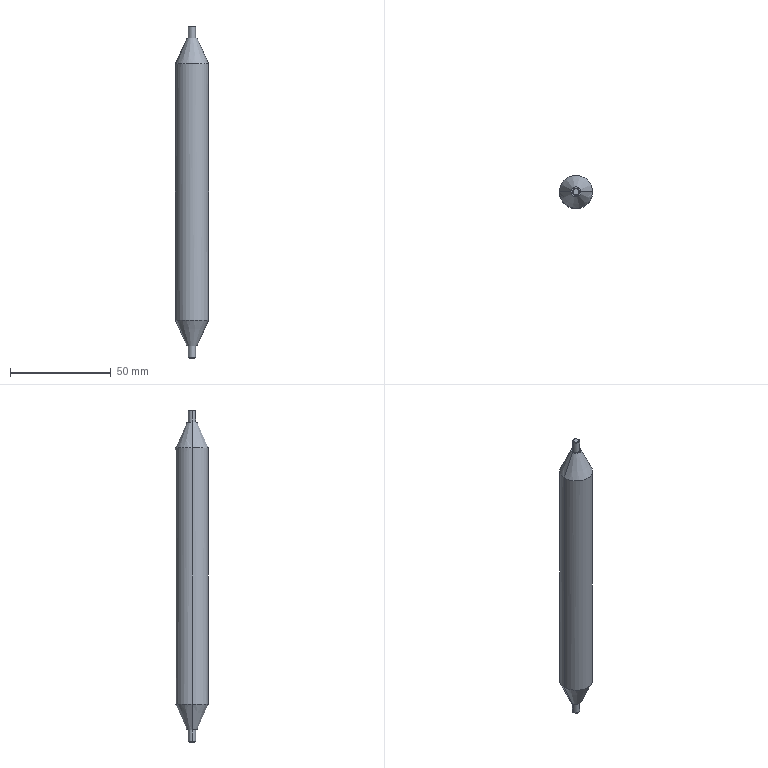Part | SolidWorks | features MirrorPattern 2, StudWizard 2, Blend 1, Extrusion 1, ICE 1 | 1 solid | 22 faces | box 16.35 x 16.35 x 164.4 mm | volume 13178 mm3 | cone 8 | cylinder 8 | plane 6 | commonest cylinder face diameters 3.5 x4 12.7 x2 16.35 x2
STEP:
#1=CARTESIAN_POINT('',(-1.414,0.,82.2));
#2=VERTEX_POINT('',#1);
#3=CARTESIAN_POINT('',(1.414,0.,82.2));
#4=VERTEX_POINT('',#3);
#5=CARTESIAN_POINT('',(0.,0.,82.2));
#6=DIRECTION('',(0.,0.,-1.));
#7=DIRECTION('',(-1.,0.,0.));
#8=AXIS2_PLACEMENT_3D('',#5,#6,#7);
#9=CIRCLE('',#8,1.414);
#10=EDGE_CURVE('',#2,#4,#9,.T.);
#11=ORIENTED_EDGE('',*,*,#10,.T.);
#12=CARTESIAN_POINT('',(1.75,0.,81.865));
#13=VERTEX_POINT('',#12);
#14=CARTESIAN_POINT('',(1.414,0.,82.2));
#15=DIRECTION('',(0.7071,0.,-0.7071));
#16=VECTOR('',#15,1000.);
#17=LINE('',#14,#16);
#18=EDGE_CURVE('',#4,#13,#17,.T.);
#19=ORIENTED_EDGE('',*,*,#18,.T.);
#20=CARTESIAN_POINT('',(-1.75,0.,81.865));
#21=VERTEX_POINT('',#20);
#22=CARTESIAN_POINT('',(0.,0.,81.865));
#23=DIRECTION('',(0.,0.,-1.));
#24=DIRECTION('',(-1.,0.,0.));
#25=AXIS2_PLACEMENT_3D('',#22,#23,#24);
#26=CIRCLE('',#25,1.75);
#27=EDGE_CURVE('',#21,#13,#26,.T.);
#28=ORIENTED_EDGE('',*,*,#27,.F.);
#29=CARTESIAN_POINT('',(-1.414,0.,82.2));
#30=DIRECTION('',(-0.7071,0.,-0.7071));
#31=VECTOR('',#30,1000.);
#32=LINE('',#29,#31);
#33=EDGE_CURVE('',#2,#21,#32,.T.);
#34=ORIENTED_EDGE('',*,*,#33,.F.);
#35=EDGE_LOOP('',(#11,#19,#28,#34));
#36=FACE_OUTER_BOUND('',#35,.T.);
#37=CARTESIAN_POINT('',(0.,0.,82.2));
#38=DIRECTION('',(0.,0.,-1.));
#39=DIRECTION('',(-1.,0.,0.));
#40=AXIS2_PLACEMENT_3D('',#37,#38,#39);
#41=CONICAL_SURFACE('',#40,1.414,0.7854);
#42=ADVANCED_FACE('',(#36),#41,.T.);
#43=ORIENTED_EDGE('',*,*,#27,.T.);
#44=CARTESIAN_POINT('',(1.75,0.,76.2));
#45=VERTEX_POINT('',#44);
#46=CARTESIAN_POINT('',(1.75,0.,82.2));
#47=DIRECTION('',(0.,0.,-1.));
#48=VECTOR('',#47,1000.);
#49=LINE('',#46,#48);
#50=EDGE_CURVE('',#13,#45,#49,.T.);
#51=ORIENTED_EDGE('',*,*,#50,.T.);
#52=CARTESIAN_POINT('',(-1.75,0.,76.2));
#53=VERTEX_POINT('',#52);
#54=CARTESIAN_POINT('',(0.,0.,76.2));
#55=DIRECTION('',(0.,0.,-1.));
#56=DIRECTION('',(-1.,0.,0.));
#57=AXIS2_PLACEMENT_3D('',#54,#55,#56);
#58=CIRCLE('',#57,1.75);
#59=EDGE_CURVE('',#53,#45,#58,.T.);
#60=ORIENTED_EDGE('',*,*,#59,.F.);
#61=CARTESIAN_POINT('',(-1.75,0.,82.2));
#62=DIRECTION('',(0.,0.,-1.));
#63=VECTOR('',#62,1000.);
#64=LINE('',#61,#63);
#65=EDGE_CURVE('',#21,#53,#64,.T.);
#66=ORIENTED_EDGE('',*,*,#65,.F.);
#67=EDGE_LOOP('',(#43,#51,#60,#66));
#68=FACE_OUTER_BOUND('',#67,.T.);
#69=CARTESIAN_POINT('',(0.,0.,82.2));
#70=DIRECTION('',(0.,0.,-1.));
#71=DIRECTION('',(-1.,0.,0.));
#72=AXIS2_PLACEMENT_3D('',#69,#70,#71);
#73=CYLINDRICAL_SURFACE('',#72,1.75);
#74=ADVANCED_FACE('',(#68),#73,.T.);
#75=CARTESIAN_POINT('',(1.414,0.,-82.2));
#76=VERTEX_POINT('',#75);
#77=CARTESIAN_POINT('',(-1.414,0.,-82.2));
#78=VERTEX_POINT('',#77);
#79=CARTESIAN_POINT('',(0.,0.,-82.2));
#80=DIRECTION('',(0.,0.,1.));
#81=DIRECTION('',(1.,0.,0.));
#82=AXIS2_PLACEMENT_3D('',#79,#80,#81);
#83=CIRCLE('',#82,1.414);
#84=EDGE_CURVE('',#76,#78,#83,.T.);
#85=ORIENTED_EDGE('',*,*,#84,.T.);
#86=CARTESIAN_POINT('',(-1.75,0.,-81.865));
#87=VERTEX_POINT('',#86);
#88=CARTESIAN_POINT('',(-1.414,0.,-82.2));
#89=DIRECTION('',(-0.7071,0.,0.7071));
#90=VECTOR('',#89,1000.);
#91=LINE('',#88,#90);
#92=EDGE_CURVE('',#78,#87,#91,.T.);
#93=ORIENTED_EDGE('',*,*,#92,.T.);
#94=CARTESIAN_POINT('',(1.75,0.,-81.865));
#95=VERTEX_POINT('',#94);
#96=CARTESIAN_POINT('',(0.,0.,-81.865));
#97=DIRECTION('',(0.,0.,1.));
#98=DIRECTION('',(1.,0.,0.));
#99=AXIS2_PLACEMENT_3D('',#96,#97,#98);
#100=CIRCLE('',#99,1.75);
#101=EDGE_CURVE('',#95,#87,#100,.T.);
#102=ORIENTED_EDGE('',*,*,#101,.F.);
#103=CARTESIAN_POINT('',(1.414,0.,-82.2));
#104=DIRECTION('',(0.7071,0.,0.7071));
#105=VECTOR('',#104,1000.);
#106=LINE('',#103,#105);
#107=EDGE_CURVE('',#76,#95,#106,.T.);
#108=ORIENTED_EDGE('',*,*,#107,.F.);
#109=EDGE_LOOP('',(#85,#93,#102,#108));
#110=FACE_OUTER_BOUND('',#109,.T.);
#111=CARTESIAN_POINT('',(0.,0.,-82.2));
#112=DIRECTION('',(0.,0.,1.));
#113=DIRECTION('',(1.,0.,0.));
#114=AXIS2_PLACEMENT_3D('',#111,#112,#113);
#115=CONICAL_SURFACE('',#114,1.414,0.7854);
#116=ADVANCED_FACE('',(#110),#115,.T.);
#117=ORIENTED_EDGE('',*,*,#101,.T.);
#118=CARTESIAN_POINT('',(-1.75,0.,-76.2));
#119=VERTEX_POINT('',#118);
#120=CARTESIAN_POINT('',(-1.75,0.,-82.2));
#121=DIRECTION('',(0.,0.,1.));
#122=VECTOR('',#121,1000.);
#123=LINE('',#120,#122);
#124=EDGE_CURVE('',#87,#119,#123,.T.);
#125=ORIENTED_EDGE('',*,*,#124,.T.);
#126=CARTESIAN_POINT('',(1.75,0.,-76.2));
#127=VERTEX_POINT('',#126);
#128=CARTESIAN_POINT('',(0.,0.,-76.2));
#129=DIRECTION('',(0.,0.,1.));
#130=DIRECTION('',(1.,0.,0.));
#131=AXIS2_PLACEMENT_3D('',#128,#129,#130);
#132=CIRCLE('',#131,1.75);
#133=EDGE_CURVE('',#127,#119,#132,.T.);
#134=ORIENTED_EDGE('',*,*,#133,.F.);
#135=CARTESIAN_POINT('',(1.75,0.,-82.2));
#136=DIRECTION('',(0.,0.,1.));
#137=VECTOR('',#136,1000.);
#138=LINE('',#135,#137);
#139=EDGE_CURVE('',#95,#127,#138,.T.);
#140=ORIENTED_EDGE('',*,*,#139,.F.);
#141=EDGE_LOOP('',(#117,#125,#134,#140));
#142=FACE_OUTER_BOUND('',#141,.T.);
#143=CARTESIAN_POINT('',(0.,0.,-82.2));
#144=DIRECTION('',(0.,0.,1.));
#145=DIRECTION('',(1.,0.,0.));
#146=AXIS2_PLACEMENT_3D('',#143,#144,#145);
#147=CYLINDRICAL_SURFACE('',#146,1.75);
#148=ADVANCED_FACE('',(#142),#147,.T.);
#149=CARTESIAN_POINT('',(2.5,0.,76.2));
#150=VERTEX_POINT('',#149);
#151=CARTESIAN_POINT('',(-2.5,0.,76.2));
#152=VERTEX_POINT('',#151);
#153=CARTESIAN_POINT('',(2.5,0.,76.2));
#154=CARTESIAN_POINT('',(2.5,-0.3272,76.2));
#155=CARTESIAN_POINT('',(2.435,-0.6544,76.2));
#156=CARTESIAN_POINT('',(2.184,-1.259,76.2));
#157=CARTESIAN_POINT('',(1.999,-1.536,76.2));
#158=CARTESIAN_POINT('',(1.536,-1.999,76.2));
#159=CARTESIAN_POINT('',(1.259,-2.184,76.2));
#160=CARTESIAN_POINT('',(0.6544,-2.435,76.2));
#161=CARTESIAN_POINT('',(0.3272,-2.5,76.2));
#162=CARTESIAN_POINT('',(-0.3272,-2.5,76.2));
#163=CARTESIAN_POINT('',(-0.6544,-2.435,76.2));
#164=CARTESIAN_POINT('',(-1.259,-2.184,76.2));
#165=CARTESIAN_POINT('',(-1.536,-1.999,76.2));
#166=CARTESIAN_POINT('',(-1.999,-1.536,76.2));
#167=CARTESIAN_POINT('',(-2.184,-1.259,76.2));
#168=CARTESIAN_POINT('',(-2.435,-0.6544,76.2));
#169=CARTESIAN_POINT('',(-2.5,-0.3272,76.2));
#170=CARTESIAN_POINT('',(-2.5,0.,76.2));
#171=B_SPLINE_CURVE_WITH_KNOTS('',3,(#153,#154,#155,#156,#157,#158,#159,#160,#161,#162,#163,#164,#165,#166,#167,#168,#169,#170),.UNSPECIFIED.,.F.,.F.,(4,2,2,2,2,2,2,2,4),(0.,0.0625,0.125,0.1875,0.25,0.3125,0.375,0.4375,0.5),.UNSPECIFIED.);
#172=EDGE_CURVE('',#150,#152,#171,.T.);
#173=ORIENTED_EDGE('',*,*,#172,.T.);
#174=CARTESIAN_POINT('',(-8.175,0.,63.5));
#175=VERTEX_POINT('',#174);
#176=CARTESIAN_POINT('',(-2.5,0.,76.2));
#177=DIRECTION('',(-0.408,0.,-0.913));
#178=VECTOR('',#177,1000.);
#179=LINE('',#176,#178);
#180=EDGE_CURVE('',#152,#175,#179,.T.);
#181=ORIENTED_EDGE('',*,*,#180,.T.);
#182=CARTESIAN_POINT('',(8.175,0.,63.5));
#183=VERTEX_POINT('',#182);
#184=CARTESIAN_POINT('',(-8.175,0.,63.5));
#185=CARTESIAN_POINT('',(-8.175,-1.07,63.5));
#186=CARTESIAN_POINT('',(-7.962,-2.14,63.5));
#187=CARTESIAN_POINT('',(-7.143,-4.117,63.5));
#188=CARTESIAN_POINT('',(-6.537,-5.024,63.5));
#189=CARTESIAN_POINT('',(-5.024,-6.537,63.5));
#190=CARTESIAN_POINT('',(-4.117,-7.143,63.5));
#191=CARTESIAN_POINT('',(-2.14,-7.962,63.5));
#192=CARTESIAN_POINT('',(-1.07,-8.175,63.5));
#193=CARTESIAN_POINT('',(1.07,-8.175,63.5));
#194=CARTESIAN_POINT('',(2.14,-7.962,63.5));
#195=CARTESIAN_POINT('',(4.117,-7.143,63.5));
#196=CARTESIAN_POINT('',(5.024,-6.537,63.5));
#197=CARTESIAN_POINT('',(6.537,-5.024,63.5));
#198=CARTESIAN_POINT('',(7.143,-4.117,63.5));
#199=CARTESIAN_POINT('',(7.962,-2.14,63.5));
#200=CARTESIAN_POINT('',(8.175,-1.07,63.5));
#201=CARTESIAN_POINT('',(8.175,0.,63.5));
#202=B_SPLINE_CURVE_WITH_KNOTS('',3,(#184,#185,#186,#187,#188,#189,#190,#191,#192,#193,#194,#195,#196,#197,#198,#199,#200,#201),.UNSPECIFIED.,.F.,.F.,(4,2,2,2,2,2,2,2,4),(0.,0.0625,0.125,0.1875,0.25,0.3125,0.375,0.4375,0.5),.UNSPECIFIED.);
#203=EDGE_CURVE('',#175,#183,#202,.T.);
#204=ORIENTED_EDGE('',*,*,#203,.T.);
#205=CARTESIAN_POINT('',(2.5,0.,76.2));
#206=DIRECTION('',(0.408,0.,-0.913));
#207=VECTOR('',#206,1000.);
#208=LINE('',#205,#207);
#209=EDGE_CURVE('',#150,#183,#208,.T.);
#210=ORIENTED_EDGE('',*,*,#209,.F.);
#211=EDGE_LOOP('',(#173,#181,#204,#210));
#212=FACE_OUTER_BOUND('',#211,.T.);
#213=CARTESIAN_POINT('',(0.,0.,76.2));
#214=DIRECTION('',(0.,0.,-1.));
#215=DIRECTION('',(1.,0.,0.));
#216=AXIS2_PLACEMENT_3D('',#213,#214,#215);
#217=CONICAL_SURFACE('',#216,2.5,0.4202);
#218=ADVANCED_FACE('',(#212),#217,.T.);
#219=CARTESIAN_POINT('',(2.5,0.,-76.2));
#220=VERTEX_POINT('',#219);
#221=CARTESIAN_POINT('',(-2.5,0.,-76.2));
#222=VERTEX_POINT('',#221);
#223=CARTESIAN_POINT('',(2.5,0.,-76.2));
#224=CARTESIAN_POINT('',(2.5,0.3272,-76.2));
#225=CARTESIAN_POINT('',(2.435,0.6544,-76.2));
#226=CARTESIAN_POINT('',(2.184,1.259,-76.2));
#227=CARTESIAN_POINT('',(1.999,1.536,-76.2));
#228=CARTESIAN_POINT('',(1.536,1.999,-76.2));
#229=CARTESIAN_POINT('',(1.259,2.184,-76.2));
#230=CARTESIAN_POINT('',(0.6544,2.435,-76.2));
#231=CARTESIAN_POINT('',(0.3272,2.5,-76.2));
#232=CARTESIAN_POINT('',(-0.3272,2.5,-76.2));
#233=CARTESIAN_POINT('',(-0.6544,2.435,-76.2));
#234=CARTESIAN_POINT('',(-1.259,2.184,-76.2));
#235=CARTESIAN_POINT('',(-1.536,1.999,-76.2));
#236=CARTESIAN_POINT('',(-1.999,1.536,-76.2));
#237=CARTESIAN_POINT('',(-2.184,1.259,-76.2));
#238=CARTESIAN_POINT('',(-2.435,0.6544,-76.2));
#239=CARTESIAN_POINT('',(-2.5,0.3272,-76.2));
#240=CARTESIAN_POINT('',(-2.5,0.,-76.2));
#241=B_SPLINE_CURVE_WITH_KNOTS('',3,(#223,#224,#225,#226,#227,#228,#229,#230,#231,#232,#233,#234,#235,#236,#237,#238,#239,#240),.UNSPECIFIED.,.F.,.F.,(4,2,2,2,2,2,2,2,4),(0.,0.0625,0.125,0.1875,0.25,0.3125,0.375,0.4375,0.5),.UNSPECIFIED.);
#242=EDGE_CURVE('',#220,#222,#241,.T.);
#243=ORIENTED_EDGE('',*,*,#242,.T.);
#244=CARTESIAN_POINT('',(-8.175,0.,-63.5));
#245=VERTEX_POINT('',#244);
#246=CARTESIAN_POINT('',(-2.5,0.,-76.2));
#247=DIRECTION('',(-0.408,0.,0.913));
#248=VECTOR('',#247,1000.);
#249=LINE('',#246,#248);
#250=EDGE_CURVE('',#222,#245,#249,.T.);
#251=ORIENTED_EDGE('',*,*,#250,.T.);
#252=CARTESIAN_POINT('',(8.175,0.,-63.5));
#253=VERTEX_POINT('',#252);
#254=CARTESIAN_POINT('',(0.,0.,-63.5));
#255=DIRECTION('',(0.,0.,-1.));
#256=DIRECTION('',(-1.,0.,0.));
#257=AXIS2_PLACEMENT_3D('',#254,#255,#256);
#258=CIRCLE('',#257,8.175);
#259=EDGE_CURVE('',#245,#253,#258,.T.);
#260=ORIENTED_EDGE('',*,*,#259,.T.);
#261=CARTESIAN_POINT('',(2.5,0.,-76.2));
#262=DIRECTION('',(0.408,0.,0.913));
#263=VECTOR('',#262,1000.);
#264=LINE('',#261,#263);
#265=EDGE_CURVE('',#220,#253,#264,.T.);
#266=ORIENTED_EDGE('',*,*,#265,.F.);
#267=EDGE_LOOP('',(#243,#251,#260,#266));
#268=FACE_OUTER_BOUND('',#267,.T.);
#269=CARTESIAN_POINT('',(0.,0.,-76.2));
#270=DIRECTION('',(0.,0.,1.));
#271=DIRECTION('',(1.,0.,0.));
#272=AXIS2_PLACEMENT_3D('',#269,#270,#271);
#273=CONICAL_SURFACE('',#272,2.5,0.4202);
#274=ADVANCED_FACE('',(#268),#273,.T.);
#275=CARTESIAN_POINT('',(8.175,0.,63.5));
#276=CARTESIAN_POINT('',(8.175,1.07,63.5));
#277=CARTESIAN_POINT('',(7.962,2.14,63.5));
#278=CARTESIAN_POINT('',(7.143,4.117,63.5));
#279=CARTESIAN_POINT('',(6.537,5.024,63.5));
#280=CARTESIAN_POINT('',(5.024,6.537,63.5));
#281=CARTESIAN_POINT('',(4.117,7.143,63.5));
#282=CARTESIAN_POINT('',(2.14,7.962,63.5));
#283=CARTESIAN_POINT('',(1.07,8.175,63.5));
#284=CARTESIAN_POINT('',(-1.07,8.175,63.5));
#285=CARTESIAN_POINT('',(-2.14,7.962,63.5));
#286=CARTESIAN_POINT('',(-4.117,7.143,63.5));
#287=CARTESIAN_POINT('',(-5.024,6.537,63.5));
#288=CARTESIAN_POINT('',(-6.537,5.024,63.5));
#289=CARTESIAN_POINT('',(-7.143,4.117,63.5));
#290=CARTESIAN_POINT('',(-7.962,2.14,63.5));
#291=CARTESIAN_POINT('',(-8.175,1.07,63.5));
#292=CARTESIAN_POINT('',(-8.175,0.,63.5));
#293=B_SPLINE_CURVE_WITH_KNOTS('',3,(#275,#276,#277,#278,#279,#280,#281,#282,#283,#284,#285,#286,#287,#288,#289,#290,#291,#292),.UNSPECIFIED.,.F.,.F.,(4,2,2,2,2,2,2,2,4),(0.5,0.5625,0.625,0.6875,0.75,0.8125,0.875,0.9375,1.),.UNSPECIFIED.);
#294=EDGE_CURVE('',#183,#175,#293,.T.);
#295=ORIENTED_EDGE('',*,*,#294,.F.);
#296=CARTESIAN_POINT('',(8.175,0.,63.5));
#297=DIRECTION('',(0.,0.,-1.));
#298=VECTOR('',#297,1000.);
#299=LINE('',#296,#298);
#300=EDGE_CURVE('',#183,#253,#299,.T.);
#301=ORIENTED_EDGE('',*,*,#300,.T.);
#302=ORIENTED_EDGE('',*,*,#259,.F.);
#303=CARTESIAN_POINT('',(-8.175,0.,63.5));
#304=DIRECTION('',(0.,0.,-1.));
#305=VECTOR('',#304,1000.);
#306=LINE('',#303,#305);
#307=EDGE_CURVE('',#175,#245,#306,.T.);
#308=ORIENTED_EDGE('',*,*,#307,.F.);
#309=EDGE_LOOP('',(#295,#301,#302,#308));
#310=FACE_OUTER_BOUND('',#309,.T.);
#311=CARTESIAN_POINT('',(0.,0.,63.5));
#312=DIRECTION('',(0.,0.,-1.));
#313=DIRECTION('',(-1.,0.,0.));
#314=AXIS2_PLACEMENT_3D('',#311,#312,#313);
#315=CYLINDRICAL_SURFACE('',#314,8.175);
#316=ADVANCED_FACE('',(#310),#315,.T.);
#317=ORIENTED_EDGE('',*,*,#300,.F.);
#318=ORIENTED_EDGE('',*,*,#203,.F.);
#319=ORIENTED_EDGE('',*,*,#307,.T.);
#320=CARTESIAN_POINT('',(0.,0.,-63.5));
#321=DIRECTION('',(0.,0.,-1.));
#322=DIRECTION('',(-1.,0.,0.));
#323=AXIS2_PLACEMENT_3D('',#320,#321,#322);
#324=CIRCLE('',#323,8.175);
#325=EDGE_CURVE('',#253,#245,#324,.T.);
#326=ORIENTED_EDGE('',*,*,#325,.F.);
#327=EDGE_LOOP('',(#317,#318,#319,#326));
#328=FACE_OUTER_BOUND('',#327,.T.);
#329=CARTESIAN_POINT('',(0.,0.,63.5));
#330=DIRECTION('',(0.,0.,-1.));
#331=DIRECTION('',(-1.,0.,0.));
#332=AXIS2_PLACEMENT_3D('',#329,#330,#331);
#333=CYLINDRICAL_SURFACE('',#332,8.175);
#334=ADVANCED_FACE('',(#328),#333,.T.);
#335=ORIENTED_EDGE('',*,*,#250,.F.);
#336=CARTESIAN_POINT('',(-2.5,0.,-76.2));
#337=CARTESIAN_POINT('',(-2.5,-0.3272,-76.2));
#338=CARTESIAN_POINT('',(-2.435,-0.6544,-76.2));
#339=CARTESIAN_POINT('',(-2.184,-1.259,-76.2));
#340=CARTESIAN_POINT('',(-1.999,-1.536,-76.2));
#341=CARTESIAN_POINT('',(-1.536,-1.999,-76.2));
#342=CARTESIAN_POINT('',(-1.259,-2.184,-76.2));
#343=CARTESIAN_POINT('',(-0.6544,-2.435,-76.2));
#344=CARTESIAN_POINT('',(-0.3272,-2.5,-76.2));
#345=CARTESIAN_POINT('',(0.3272,-2.5,-76.2));
#346=CARTESIAN_POINT('',(0.6544,-2.435,-76.2));
#347=CARTESIAN_POINT('',(1.259,-2.184,-76.2));
#348=CARTESIAN_POINT('',(1.536,-1.999,-76.2));
#349=CARTESIAN_POINT('',(1.999,-1.536,-76.2));
#350=CARTESIAN_POINT('',(2.184,-1.259,-76.2));
#351=CARTESIAN_POINT('',(2.435,-0.6544,-76.2));
#352=CARTESIAN_POINT('',(2.5,-0.3272,-76.2));
#353=CARTESIAN_POINT('',(2.5,0.,-76.2));
#354=B_SPLINE_CURVE_WITH_KNOTS('',3,(#336,#337,#338,#339,#340,#341,#342,#343,#344,#345,#346,#347,#348,#349,#350,#351,#352,#353),.UNSPECIFIED.,.F.,.F.,(4,2,2,2,2,2,2,2,4),(0.5,0.5625,0.625,0.6875,0.75,0.8125,0.875,0.9375,1.),.UNSPECIFIED.);
#355=EDGE_CURVE('',#222,#220,#354,.T.);
#356=ORIENTED_EDGE('',*,*,#355,.T.);
#357=ORIENTED_EDGE('',*,*,#265,.T.);
#358=ORIENTED_EDGE('',*,*,#325,.T.);
#359=EDGE_LOOP('',(#335,#356,#357,#358));
#360=FACE_OUTER_BOUND('',#359,.T.);
#361=CARTESIAN_POINT('',(0.,0.,-76.2));
#362=DIRECTION('',(0.,0.,1.));
#363=DIRECTION('',(1.,0.,0.));
#364=AXIS2_PLACEMENT_3D('',#361,#362,#363);
#365=CONICAL_SURFACE('',#364,2.5,0.4202);
#366=ADVANCED_FACE('',(#360),#365,.T.);
#367=ORIENTED_EDGE('',*,*,#180,.F.);
#368=CARTESIAN_POINT('',(-2.5,0.,76.2));
#369=CARTESIAN_POINT('',(-2.5,0.3272,76.2));
#370=CARTESIAN_POINT('',(-2.435,0.6544,76.2));
#371=CARTESIAN_POINT('',(-2.184,1.259,76.2));
#372=CARTESIAN_POINT('',(-1.999,1.536,76.2));
#373=CARTESIAN_POINT('',(-1.536,1.999,76.2));
#374=CARTESIAN_POINT('',(-1.259,2.184,76.2));
#375=CARTESIAN_POINT('',(-0.6544,2.435,76.2));
#376=CARTESIAN_POINT('',(-0.3272,2.5,76.2));
#377=CARTESIAN_POINT('',(0.3272,2.5,76.2));
#378=CARTESIAN_POINT('',(0.6544,2.435,76.2));
#379=CARTESIAN_POINT('',(1.259,2.184,76.2));
#380=CARTESIAN_POINT('',(1.536,1.999,76.2));
#381=CARTESIAN_POINT('',(1.999,1.536,76.2));
#382=CARTESIAN_POINT('',(2.184,1.259,76.2));
#383=CARTESIAN_POINT('',(2.435,0.6544,76.2));
#384=CARTESIAN_POINT('',(2.5,0.3272,76.2));
#385=CARTESIAN_POINT('',(2.5,0.,76.2));
#386=B_SPLINE_CURVE_WITH_KNOTS('',3,(#368,#369,#370,#371,#372,#373,#374,#375,#376,#377,#378,#379,#380,#381,#382,#383,#384,#385),.UNSPECIFIED.,.F.,.F.,(4,2,2,2,2,2,2,2,4),(0.5,0.5625,0.625,0.6875,0.75,0.8125,0.875,0.9375,1.),.UNSPECIFIED.);
#387=EDGE_CURVE('',#152,#150,#386,.T.);
#388=ORIENTED_EDGE('',*,*,#387,.T.);
#389=ORIENTED_EDGE('',*,*,#209,.T.);
#390=ORIENTED_EDGE('',*,*,#294,.T.);
#391=EDGE_LOOP('',(#367,#388,#389,#390));
#392=FACE_OUTER_BOUND('',#391,.T.);
#393=CARTESIAN_POINT('',(0.,0.,76.2));
#394=DIRECTION('',(0.,0.,-1.));
#395=DIRECTION('',(1.,0.,0.));
#396=AXIS2_PLACEMENT_3D('',#393,#394,#395);
#397=CONICAL_SURFACE('',#396,2.5,0.4202);
#398=ADVANCED_FACE('',(#392),#397,.T.);
#399=ORIENTED_EDGE('',*,*,#124,.F.);
#400=CARTESIAN_POINT('',(0.,0.,-81.865));
#401=DIRECTION('',(0.,0.,1.));
#402=DIRECTION('',(1.,0.,0.));
#403=AXIS2_PLACEMENT_3D('',#400,#401,#402);
#404=CIRCLE('',#403,1.75);
#405=EDGE_CURVE('',#87,#95,#404,.T.);
#406=ORIENTED_EDGE('',*,*,#405,.T.);
#407=ORIENTED_EDGE('',*,*,#139,.T.);
#408=CARTESIAN_POINT('',(0.,0.,-76.2));
#409=DIRECTION('',(0.,0.,1.));
#410=DIRECTION('',(1.,0.,0.));
#411=AXIS2_PLACEMENT_3D('',#408,#409,#410);
#412=CIRCLE('',#411,1.75);
#413=EDGE_CURVE('',#119,#127,#412,.T.);
#414=ORIENTED_EDGE('',*,*,#413,.F.);
#415=EDGE_LOOP('',(#399,#406,#407,#414));
#416=FACE_OUTER_BOUND('',#415,.T.);
#417=CARTESIAN_POINT('',(0.,0.,-82.2));
#418=DIRECTION('',(0.,0.,1.));
#419=DIRECTION('',(1.,0.,0.));
#420=AXIS2_PLACEMENT_3D('',#417,#418,#419);
#421=CYLINDRICAL_SURFACE('',#420,1.75);
#422=ADVANCED_FACE('',(#416),#421,.T.);
#423=ORIENTED_EDGE('',*,*,#242,.F.);
#424=ORIENTED_EDGE('',*,*,#355,.F.);
#425=EDGE_LOOP('',(#423,#424));
#426=FACE_OUTER_BOUND('',#425,.T.);
#427=ORIENTED_EDGE('',*,*,#133,.T.);
#428=ORIENTED_EDGE('',*,*,#413,.T.);
#429=EDGE_LOOP('',(#427,#428));
#430=FACE_BOUND('',#429,.T.);
#431=CARTESIAN_POINT('',(1.75,0.,-76.2));
#432=DIRECTION('',(0.,0.,1.));
#433=DIRECTION('',(1.,0.,0.));
#434=AXIS2_PLACEMENT_3D('',#431,#432,#433);
#435=PLANE('',#434);
#436=ADVANCED_FACE('',(#426,#430),#435,.F.);
#437=ORIENTED_EDGE('',*,*,#92,.F.);
#438=CARTESIAN_POINT('',(0.,0.,-82.2));
#439=DIRECTION('',(0.,0.,1.));
#440=DIRECTION('',(1.,0.,0.));
#441=AXIS2_PLACEMENT_3D('',#438,#439,#440);
#442=CIRCLE('',#441,1.414);
#443=EDGE_CURVE('',#78,#76,#442,.T.);
#444=ORIENTED_EDGE('',*,*,#443,.T.);
#445=ORIENTED_EDGE('',*,*,#107,.T.);
#446=ORIENTED_EDGE('',*,*,#405,.F.);
#447=EDGE_LOOP('',(#437,#444,#445,#446));
#448=FACE_OUTER_BOUND('',#447,.T.);
#449=CARTESIAN_POINT('',(0.,0.,-82.2));
#450=DIRECTION('',(0.,0.,1.));
#451=DIRECTION('',(1.,0.,0.));
#452=AXIS2_PLACEMENT_3D('',#449,#450,#451);
#453=CONICAL_SURFACE('',#452,1.414,0.7854);
#454=ADVANCED_FACE('',(#448),#453,.T.);
#455=ORIENTED_EDGE('',*,*,#84,.F.);
#456=ORIENTED_EDGE('',*,*,#443,.F.);
#457=EDGE_LOOP('',(#455,#456));
#458=FACE_OUTER_BOUND('',#457,.T.);
#459=CARTESIAN_POINT('',(0.,0.,-82.2));
#460=DIRECTION('',(0.,0.,-1.));
#461=DIRECTION('',(-1.,0.,0.));
#462=AXIS2_PLACEMENT_3D('',#459,#460,#461);
#463=PLANE('',#462);
#464=ADVANCED_FACE('',(#458),#463,.T.);
#465=ORIENTED_EDGE('',*,*,#50,.F.);
#466=CARTESIAN_POINT('',(0.,0.,81.865));
#467=DIRECTION('',(0.,0.,-1.));
#468=DIRECTION('',(-1.,0.,0.));
#469=AXIS2_PLACEMENT_3D('',#466,#467,#468);
#470=CIRCLE('',#469,1.75);
#471=EDGE_CURVE('',#13,#21,#470,.T.);
#472=ORIENTED_EDGE('',*,*,#471,.T.);
#473=ORIENTED_EDGE('',*,*,#65,.T.);
#474=CARTESIAN_POINT('',(0.,0.,76.2));
#475=DIRECTION('',(0.,0.,-1.));
#476=DIRECTION('',(-1.,0.,0.));
#477=AXIS2_PLACEMENT_3D('',#474,#475,#476);
#478=CIRCLE('',#477,1.75);
#479=EDGE_CURVE('',#45,#53,#478,.T.);
#480=ORIENTED_EDGE('',*,*,#479,.F.);
#481=EDGE_LOOP('',(#465,#472,#473,#480));
#482=FACE_OUTER_BOUND('',#481,.T.);
#483=CARTESIAN_POINT('',(0.,0.,82.2));
#484=DIRECTION('',(0.,0.,-1.));
#485=DIRECTION('',(-1.,0.,0.));
#486=AXIS2_PLACEMENT_3D('',#483,#484,#485);
#487=CYLINDRICAL_SURFACE('',#486,1.75);
#488=ADVANCED_FACE('',(#482),#487,.T.);
#489=ORIENTED_EDGE('',*,*,#172,.F.);
#490=ORIENTED_EDGE('',*,*,#387,.F.);
#491=EDGE_LOOP('',(#489,#490));
#492=FACE_OUTER_BOUND('',#491,.T.);
#493=ORIENTED_EDGE('',*,*,#59,.T.);
#494=ORIENTED_EDGE('',*,*,#479,.T.);
#495=EDGE_LOOP('',(#493,#494));
#496=FACE_BOUND('',#495,.T.);
#497=CARTESIAN_POINT('',(1.75,0.,76.2));
#498=DIRECTION('',(0.,0.,-1.));
#499=DIRECTION('',(-1.,0.,0.));
#500=AXIS2_PLACEMENT_3D('',#497,#498,#499);
#501=PLANE('',#500);
#502=ADVANCED_FACE('',(#492,#496),#501,.F.);
#503=ORIENTED_EDGE('',*,*,#18,.F.);
#504=CARTESIAN_POINT('',(0.,0.,82.2));
#505=DIRECTION('',(0.,0.,-1.));
#506=DIRECTION('',(-1.,0.,0.));
#507=AXIS2_PLACEMENT_3D('',#504,#505,#506);
#508=CIRCLE('',#507,1.414);
#509=EDGE_CURVE('',#4,#2,#508,.T.);
#510=ORIENTED_EDGE('',*,*,#509,.T.);
#511=ORIENTED_EDGE('',*,*,#33,.T.);
#512=ORIENTED_EDGE('',*,*,#471,.F.);
#513=EDGE_LOOP('',(#503,#510,#511,#512));
#514=FACE_OUTER_BOUND('',#513,.T.);
#515=CARTESIAN_POINT('',(0.,0.,82.2));
#516=DIRECTION('',(0.,0.,-1.));
#517=DIRECTION('',(-1.,0.,0.));
#518=AXIS2_PLACEMENT_3D('',#515,#516,#517);
#519=CONICAL_SURFACE('',#518,1.414,0.7854);
#520=ADVANCED_FACE('',(#514),#519,.T.);
#521=ORIENTED_EDGE('',*,*,#10,.F.);
#522=ORIENTED_EDGE('',*,*,#509,.F.);
#523=EDGE_LOOP('',(#521,#522));
#524=FACE_OUTER_BOUND('',#523,.T.);
#525=CARTESIAN_POINT('',(0.,0.,82.2));
#526=DIRECTION('',(0.,0.,1.));
#527=DIRECTION('',(-1.,0.,0.));
#528=AXIS2_PLACEMENT_3D('',#525,#526,#527);
#529=PLANE('',#528);
#530=ADVANCED_FACE('',(#524),#529,.T.);
#531=CLOSED_SHELL('',(#42,#74,#116,#148,#218,#274,#316,#334,#366,#398,#422,#436,#454,#464,#488,#502,#520,#530));
#532=CARTESIAN_POINT('',(-6.35,0.,63.5));
#533=VERTEX_POINT('',#532);
#534=CARTESIAN_POINT('',(6.35,0.,63.5));
#535=VERTEX_POINT('',#534);
#536=CARTESIAN_POINT('',(0.,0.,63.5));
#537=DIRECTION('',(0.,0.,1.));
#538=DIRECTION('',(1.,0.,0.));
#539=AXIS2_PLACEMENT_3D('',#536,#537,#538);
#540=CIRCLE('',#539,6.35);
#541=EDGE_CURVE('',#533,#535,#540,.T.);
#542=ORIENTED_EDGE('',*,*,#541,.T.);
#543=CARTESIAN_POINT('',(6.35,0.,-63.5));
#544=VERTEX_POINT('',#543);
#545=CARTESIAN_POINT('',(6.35,0.,63.5));
#546=DIRECTION('',(0.,0.,-1.));
#547=VECTOR('',#546,1000.);
#548=LINE('',#545,#547);
#549=EDGE_CURVE('',#535,#544,#548,.T.);
#550=ORIENTED_EDGE('',*,*,#549,.T.);
#551=CARTESIAN_POINT('',(-6.35,0.,-63.5));
#552=VERTEX_POINT('',#551);
#553=CARTESIAN_POINT('',(0.,0.,-63.5));
#554=DIRECTION('',(0.,0.,1.));
#555=DIRECTION('',(1.,0.,0.));
#556=AXIS2_PLACEMENT_3D('',#553,#554,#555);
#557=CIRCLE('',#556,6.35);
#558=EDGE_CURVE('',#552,#544,#557,.T.);
#559=ORIENTED_EDGE('',*,*,#558,.F.);
#560=CARTESIAN_POINT('',(-6.35,0.,63.5));
#561=DIRECTION('',(0.,0.,-1.));
#562=VECTOR('',#561,1000.);
#563=LINE('',#560,#562);
#564=EDGE_CURVE('',#533,#552,#563,.T.);
#565=ORIENTED_EDGE('',*,*,#564,.F.);
#566=EDGE_LOOP('',(#542,#550,#559,#565));
#567=FACE_OUTER_BOUND('',#566,.T.);
#568=CARTESIAN_POINT('',(0.,0.,63.5));
#569=DIRECTION('',(0.,0.,-1.));
#570=DIRECTION('',(-1.,0.,0.));
#571=AXIS2_PLACEMENT_3D('',#568,#569,#570);
#572=CYLINDRICAL_SURFACE('',#571,6.35);
#573=ADVANCED_FACE('',(#567),#572,.F.);
#574=ORIENTED_EDGE('',*,*,#558,.T.);
#575=CARTESIAN_POINT('',(0.,0.,-63.5));
#576=DIRECTION('',(0.,0.,1.));
#577=DIRECTION('',(1.,0.,0.));
#578=AXIS2_PLACEMENT_3D('',#575,#576,#577);
#579=CIRCLE('',#578,6.35);
#580=EDGE_CURVE('',#544,#552,#579,.T.);
#581=ORIENTED_EDGE('',*,*,#580,.T.);
#582=EDGE_LOOP('',(#574,#581));
#583=FACE_OUTER_BOUND('',#582,.T.);
#584=CARTESIAN_POINT('',(0.,0.,-63.5));
#585=DIRECTION('',(0.,0.,-1.));
#586=DIRECTION('',(-1.,0.,0.));
#587=AXIS2_PLACEMENT_3D('',#584,#585,#586);
#588=PLANE('',#587);
#589=ADVANCED_FACE('',(#583),#588,.F.);
#590=ORIENTED_EDGE('',*,*,#549,.F.);
#591=CARTESIAN_POINT('',(0.,0.,63.5));
#592=DIRECTION('',(0.,0.,1.));
#593=DIRECTION('',(1.,0.,0.));
#594=AXIS2_PLACEMENT_3D('',#591,#592,#593);
#595=CIRCLE('',#594,6.35);
#596=EDGE_CURVE('',#535,#533,#595,.T.);
#597=ORIENTED_EDGE('',*,*,#596,.T.);
#598=ORIENTED_EDGE('',*,*,#564,.T.);
#599=ORIENTED_EDGE('',*,*,#580,.F.);
#600=EDGE_LOOP('',(#590,#597,#598,#599));
#601=FACE_OUTER_BOUND('',#600,.T.);
#602=CARTESIAN_POINT('',(0.,0.,63.5));
#603=DIRECTION('',(0.,0.,-1.));
#604=DIRECTION('',(-1.,0.,0.));
#605=AXIS2_PLACEMENT_3D('',#602,#603,#604);
#606=CYLINDRICAL_SURFACE('',#605,6.35);
#607=ADVANCED_FACE('',(#601),#606,.F.);
#608=ORIENTED_EDGE('',*,*,#541,.F.);
#609=ORIENTED_EDGE('',*,*,#596,.F.);
#610=EDGE_LOOP('',(#608,#609));
#611=FACE_OUTER_BOUND('',#610,.T.);
#612=CARTESIAN_POINT('',(0.,0.,63.5));
#613=DIRECTION('',(0.,0.,1.));
#614=DIRECTION('',(-1.,0.,0.));
#615=AXIS2_PLACEMENT_3D('',#612,#613,#614);
#616=PLANE('',#615);
#617=ADVANCED_FACE('',(#611),#616,.F.);
#618=CLOSED_SHELL('',(#573,#589,#607,#617));
#619=ORIENTED_CLOSED_SHELL('',*,#618,.F.);
#620=BREP_WITH_VOIDS('',#531,(#619));
#621=CARTESIAN_POINT('',(0.,0.,0.));
#622=DIRECTION('',(0.,0.,1.));
#623=DIRECTION('',(1.,0.,0.));
#624=AXIS2_PLACEMENT_3D('',#621,#622,#623);
#625=(LENGTH_UNIT()NAMED_UNIT(*)SI_UNIT(.MILLI.,.METRE.));
#626=UNCERTAINTY_MEASURE_WITH_UNIT(LENGTH_MEASURE(0.00001),#625,'','');
#627=(NAMED_UNIT(*)PLANE_ANGLE_UNIT()SI_UNIT($,.RADIAN.));
#628=(NAMED_UNIT(*)SI_UNIT($,.STERADIAN.)SOLID_ANGLE_UNIT());
#629=(GEOMETRIC_REPRESENTATION_CONTEXT(3)GLOBAL_UNCERTAINTY_ASSIGNED_CONTEXT((#626))GLOBAL_UNIT_ASSIGNED_CONTEXT((#625,#627,#628))REPRESENTATION_CONTEXT('',''));
#630=ADVANCED_BREP_SHAPE_REPRESENTATION('',(#620,#624),#629);